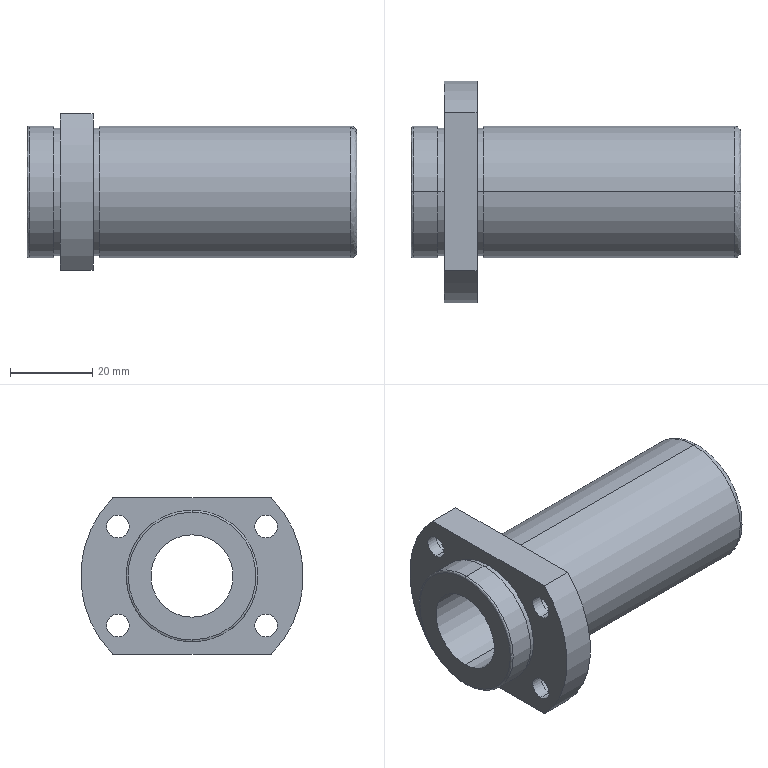Part | STEP file | Guided double-liner flanged linear bearing LML21-d20 | 1 solid | 44 faces | box 80 x 54 x 38 mm | volume 45928 mm3 | cylinder 28 | plane 12 | spline 4 | commonest cylinder face diameters 5.5 x8 9 x8 31 x4 32 x4 20 x2 54 x2